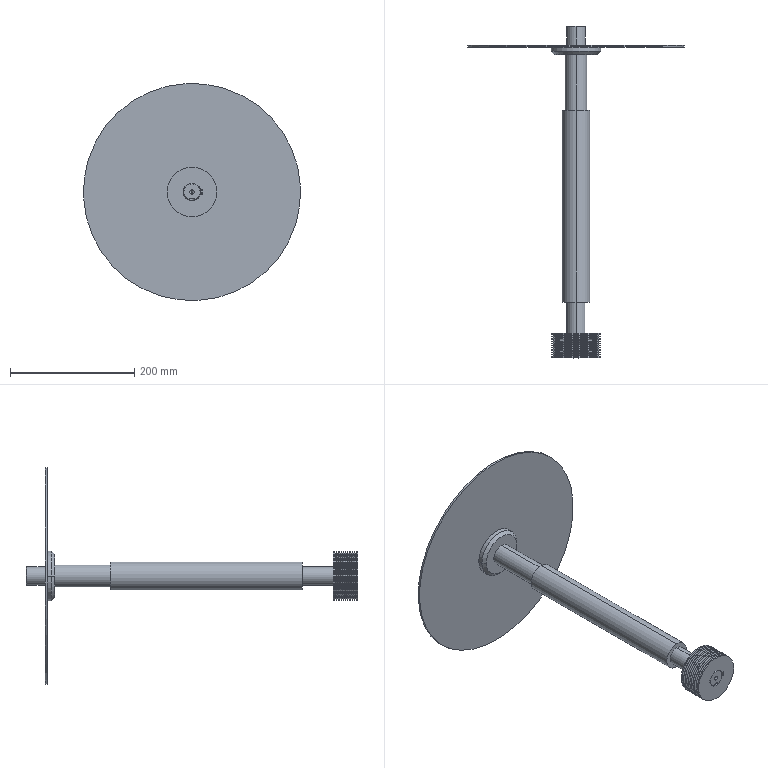Part | SolidWorks | 4 solids | 218 faces | box 350 x 535 x 350 mm | volume 1155640 mm3 | torus 80 | cylinder 70 | cone 48 | plane 20 | commonest cylinder face diameters 80 x24 73.1 x20 30 x6 28 x5 50 x4 7 x2